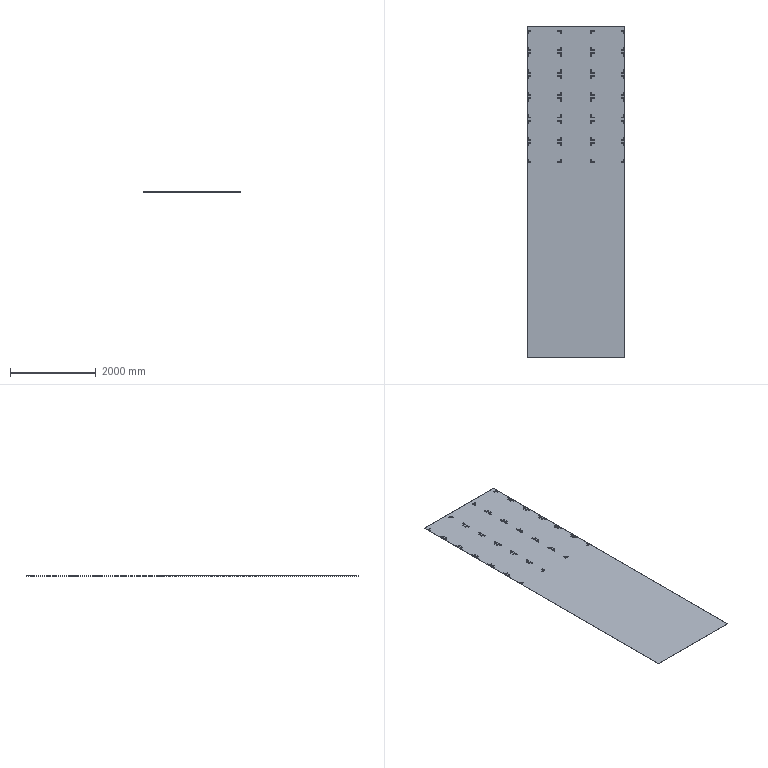Part | STEP file | 750078135 | 1 solid | 966 faces | box 2272 x 7726 x 4 mm | volume 69829888 mm3 | plane 966